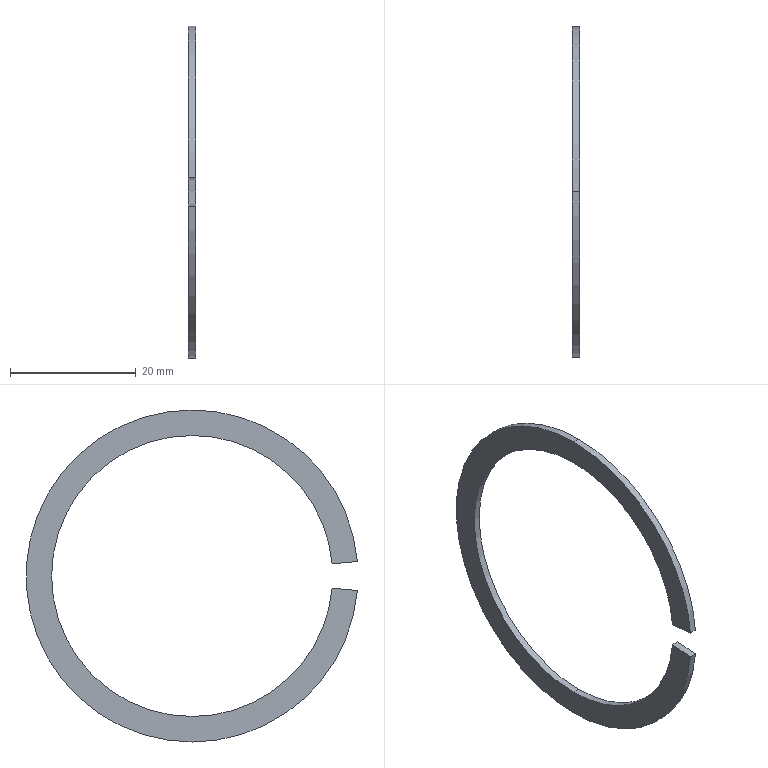Part | STEP file | 0229_Z_B6204ZZNR_2 | 1 solid | 10 faces | box 1.12 x 52.6 x 52.7 mm | volume 674.018 mm3 | cylinder 6 | plane 4 | commonest cylinder face diameters 44.6 x3 52.7 x3
STEP:
#1=CARTESIAN_POINT('',(0.,0.,0.));
#2=DIRECTION('',(0.,0.,1.));
#3=DIRECTION('',(1.,0.,0.));
#4=AXIS2_PLACEMENT_3D('',#1,#2,#3);
#5=CARTESIAN_POINT('',(3.58,-22.215,-1.944));
#6=VERTEX_POINT('',#5);
#7=CARTESIAN_POINT('',(2.46,-22.215,-1.944));
#8=VERTEX_POINT('',#7);
#9=CARTESIAN_POINT('',(2.46,-22.215,-1.944));
#10=DIRECTION('',(-1.,0.,0.));
#11=VECTOR('',#10,1.);
#12=LINE('',#9,#11);
#13=CARTESIAN_POINT('',(2.46,0.,0.));
#14=DIRECTION('',(-1.,0.,0.));
#15=DIRECTION('',(0.,0.,1.));
#16=AXIS2_PLACEMENT_3D('',#13,#14,#15);
#17=CYLINDRICAL_SURFACE('',#16,22.3);
#18=CARTESIAN_POINT('',(4.625,0.));
#19=DIRECTION('',(0.,1.));
#20=VECTOR('',#19,1.);
#21=LINE('',#18,#20);
#22=(GEOMETRIC_REPRESENTATION_CONTEXT(2)PARAMETRIC_REPRESENTATION_CONTEXT()REPRESENTATION_CONTEXT('',''));
#23=DEFINITIONAL_REPRESENTATION('',(#21),#22);
#24=PCURVE('',#17,#23);
#25=CARTESIAN_POINT('',(2.46,-26.25,-2.297));
#26=DIRECTION('',(0.,-0.08716,0.9962));
#27=DIRECTION('',(0.,-0.9962,-0.08716));
#28=AXIS2_PLACEMENT_3D('',#25,#26,#27);
#29=PLANE('',#28);
#30=CARTESIAN_POINT('',(-4.05,0.));
#31=DIRECTION('',(0.,-1.));
#32=VECTOR('',#31,1.);
#33=LINE('',#30,#32);
#34=(GEOMETRIC_REPRESENTATION_CONTEXT(2)PARAMETRIC_REPRESENTATION_CONTEXT()REPRESENTATION_CONTEXT('',''));
#35=DEFINITIONAL_REPRESENTATION('',(#33),#34);
#36=PCURVE('',#29,#35);
#37=SURFACE_CURVE('',#12,(#24,#36),.PCURVE_S1.);
#38=EDGE_CURVE('',#6,#8,#37,.T.);
#39=ORIENTED_EDGE('',*,*,#38,.T.);
#40=CARTESIAN_POINT('',(2.46,0.,-22.3));
#41=VERTEX_POINT('',#40);
#42=CARTESIAN_POINT('',(2.46,0.,0.));
#43=DIRECTION('',(1.,0.,0.));
#44=DIRECTION('',(0.,0.,1.));
#45=AXIS2_PLACEMENT_3D('',#42,#43,#44);
#46=CIRCLE('',#45,22.3);
#47=CARTESIAN_POINT('',(6.283,0.));
#48=DIRECTION('',(-1.,0.));
#49=VECTOR('',#48,1.);
#50=LINE('',#47,#49);
#51=(GEOMETRIC_REPRESENTATION_CONTEXT(2)PARAMETRIC_REPRESENTATION_CONTEXT()REPRESENTATION_CONTEXT('',''));
#52=DEFINITIONAL_REPRESENTATION('',(#50),#51);
#53=PCURVE('',#17,#52);
#54=CARTESIAN_POINT('',(2.46,0.,0.));
#55=DIRECTION('',(1.,0.,0.));
#56=DIRECTION('',(0.,0.,-1.));
#57=AXIS2_PLACEMENT_3D('',#54,#55,#56);
#58=PLANE('',#57);
#59=CARTESIAN_POINT('',(0.,0.));
#60=DIRECTION('',(-1.,0.));
#61=AXIS2_PLACEMENT_2D('',#59,#60);
#62=CIRCLE('',#61,22.3);
#63=(GEOMETRIC_REPRESENTATION_CONTEXT(2)PARAMETRIC_REPRESENTATION_CONTEXT()REPRESENTATION_CONTEXT('',''));
#64=DEFINITIONAL_REPRESENTATION('',(#62),#63);
#65=PCURVE('',#58,#64);
#66=SURFACE_CURVE('',#46,(#53,#65),.PCURVE_S1.);
#67=EDGE_CURVE('',#8,#41,#66,.T.);
#68=ORIENTED_EDGE('',*,*,#67,.T.);
#69=CARTESIAN_POINT('',(3.58,0.,-22.3));
#70=VERTEX_POINT('',#69);
#71=CARTESIAN_POINT('',(2.46,0.,-22.3));
#72=DIRECTION('',(-1.,0.,0.));
#73=VECTOR('',#72,1.);
#74=LINE('',#71,#73);
#75=CARTESIAN_POINT('',(3.142,0.));
#76=DIRECTION('',(0.,1.));
#77=VECTOR('',#76,1.);
#78=LINE('',#75,#77);
#79=(GEOMETRIC_REPRESENTATION_CONTEXT(2)PARAMETRIC_REPRESENTATION_CONTEXT()REPRESENTATION_CONTEXT('',''));
#80=DEFINITIONAL_REPRESENTATION('',(#78),#79);
#81=PCURVE('',#17,#80);
#82=CARTESIAN_POINT('',(2.46,0.,0.));
#83=DIRECTION('',(-1.,0.,0.));
#84=DIRECTION('',(0.,0.,1.));
#85=AXIS2_PLACEMENT_3D('',#82,#83,#84);
#86=CYLINDRICAL_SURFACE('',#85,22.3);
#87=CARTESIAN_POINT('',(3.142,0.));
#88=DIRECTION('',(0.,1.));
#89=VECTOR('',#88,1.);
#90=LINE('',#87,#89);
#91=(GEOMETRIC_REPRESENTATION_CONTEXT(2)PARAMETRIC_REPRESENTATION_CONTEXT()REPRESENTATION_CONTEXT('',''));
#92=DEFINITIONAL_REPRESENTATION('',(#90),#91);
#93=PCURVE('',#86,#92);
#94=SURFACE_CURVE('',#74,(#81,#93),.PCURVE_S1.);
#95=EDGE_CURVE('',#70,#41,#94,.T.);
#96=ORIENTED_EDGE('',*,*,#95,.F.);
#97=CARTESIAN_POINT('',(3.58,0.,0.));
#98=DIRECTION('',(-1.,0.,0.));
#99=DIRECTION('',(0.,0.,1.));
#100=AXIS2_PLACEMENT_3D('',#97,#98,#99);
#101=CIRCLE('',#100,22.3);
#102=CARTESIAN_POINT('',(0.,-1.12));
#103=DIRECTION('',(1.,0.));
#104=VECTOR('',#103,1.);
#105=LINE('',#102,#104);
#106=(GEOMETRIC_REPRESENTATION_CONTEXT(2)PARAMETRIC_REPRESENTATION_CONTEXT()REPRESENTATION_CONTEXT('',''));
#107=DEFINITIONAL_REPRESENTATION('',(#105),#106);
#108=PCURVE('',#17,#107);
#109=CARTESIAN_POINT('',(3.58,0.,0.));
#110=DIRECTION('',(1.,0.,0.));
#111=DIRECTION('',(0.,0.,-1.));
#112=AXIS2_PLACEMENT_3D('',#109,#110,#111);
#113=PLANE('',#112);
#114=CARTESIAN_POINT('',(-22.3,0.));
#115=CARTESIAN_POINT('',(-22.3,38.625));
#116=CARTESIAN_POINT('',(11.15,19.312));
#117=CARTESIAN_POINT('',(44.6,0.));
#118=CARTESIAN_POINT('',(11.15,-19.312));
#119=CARTESIAN_POINT('',(-22.3,-38.625));
#120=CARTESIAN_POINT('',(-22.3,0.));
#121=(BOUNDED_CURVE()B_SPLINE_CURVE(2,(#114,#115,#116,#117,#118,#119,#120),.UNSPECIFIED.,.T.,.F.)B_SPLINE_CURVE_WITH_KNOTS((1,2,2,2,2,1),(-2.094,0.,2.094,4.189,6.283,8.378),.UNSPECIFIED.)CURVE()GEOMETRIC_REPRESENTATION_ITEM()RATIONAL_B_SPLINE_CURVE((1.,0.5,1.,0.5,1.,0.5,1.))REPRESENTATION_ITEM(''));
#122=(GEOMETRIC_REPRESENTATION_CONTEXT(2)PARAMETRIC_REPRESENTATION_CONTEXT()REPRESENTATION_CONTEXT('',''));
#123=DEFINITIONAL_REPRESENTATION('',(#121),#122);
#124=PCURVE('',#113,#123);
#125=SURFACE_CURVE('',#101,(#108,#124),.PCURVE_S1.);
#126=EDGE_CURVE('',#70,#6,#125,.T.);
#127=ORIENTED_EDGE('',*,*,#126,.T.);
#128=EDGE_LOOP('',(#39,#68,#96,#127));
#129=FACE_BOUND('',#128,.F.);
#130=ADVANCED_FACE('',(#129),#17,.F.);
#131=CARTESIAN_POINT('',(2.46,0.,22.3));
#132=VERTEX_POINT('',#131);
#133=CARTESIAN_POINT('',(2.46,0.,0.));
#134=DIRECTION('',(1.,0.,0.));
#135=DIRECTION('',(0.,0.,1.));
#136=AXIS2_PLACEMENT_3D('',#133,#134,#135);
#137=CIRCLE('',#136,22.3);
#138=CARTESIAN_POINT('',(6.283,0.));
#139=DIRECTION('',(-1.,0.));
#140=VECTOR('',#139,1.);
#141=LINE('',#138,#140);
#142=(GEOMETRIC_REPRESENTATION_CONTEXT(2)PARAMETRIC_REPRESENTATION_CONTEXT()REPRESENTATION_CONTEXT('',''));
#143=DEFINITIONAL_REPRESENTATION('',(#141),#142);
#144=PCURVE('',#86,#143);
#145=CARTESIAN_POINT('',(0.,0.));
#146=DIRECTION('',(-1.,0.));
#147=AXIS2_PLACEMENT_2D('',#145,#146);
#148=CIRCLE('',#147,22.3);
#149=(GEOMETRIC_REPRESENTATION_CONTEXT(2)PARAMETRIC_REPRESENTATION_CONTEXT()REPRESENTATION_CONTEXT('',''));
#150=DEFINITIONAL_REPRESENTATION('',(#148),#149);
#151=PCURVE('',#58,#150);
#152=SURFACE_CURVE('',#137,(#144,#151),.PCURVE_S1.);
#153=EDGE_CURVE('',#41,#132,#152,.T.);
#154=ORIENTED_EDGE('',*,*,#153,.T.);
#155=CARTESIAN_POINT('',(3.58,0.,22.3));
#156=VERTEX_POINT('',#155);
#157=CARTESIAN_POINT('',(2.46,0.,22.3));
#158=DIRECTION('',(-1.,0.,0.));
#159=VECTOR('',#158,1.);
#160=LINE('',#157,#159);
#161=CARTESIAN_POINT('',(0.,0.));
#162=DIRECTION('',(0.,1.));
#163=VECTOR('',#162,1.);
#164=LINE('',#161,#163);
#165=(GEOMETRIC_REPRESENTATION_CONTEXT(2)PARAMETRIC_REPRESENTATION_CONTEXT()REPRESENTATION_CONTEXT('',''));
#166=DEFINITIONAL_REPRESENTATION('',(#164),#165);
#167=PCURVE('',#86,#166);
#168=CARTESIAN_POINT('',(2.46,0.,0.));
#169=DIRECTION('',(-1.,0.,0.));
#170=DIRECTION('',(0.,0.,1.));
#171=AXIS2_PLACEMENT_3D('',#168,#169,#170);
#172=CYLINDRICAL_SURFACE('',#171,22.3);
#173=CARTESIAN_POINT('',(6.283,0.));
#174=DIRECTION('',(0.,1.));
#175=VECTOR('',#174,1.);
#176=LINE('',#173,#175);
#177=(GEOMETRIC_REPRESENTATION_CONTEXT(2)PARAMETRIC_REPRESENTATION_CONTEXT()REPRESENTATION_CONTEXT('',''));
#178=DEFINITIONAL_REPRESENTATION('',(#176),#177);
#179=PCURVE('',#172,#178);
#180=SURFACE_CURVE('',#160,(#167,#179),.PCURVE_S1.);
#181=EDGE_CURVE('',#156,#132,#180,.T.);
#182=ORIENTED_EDGE('',*,*,#181,.F.);
#183=CARTESIAN_POINT('',(3.58,0.,0.));
#184=DIRECTION('',(-1.,0.,0.));
#185=DIRECTION('',(0.,0.,1.));
#186=AXIS2_PLACEMENT_3D('',#183,#184,#185);
#187=CIRCLE('',#186,22.3);
#188=CARTESIAN_POINT('',(0.,-1.12));
#189=DIRECTION('',(1.,0.));
#190=VECTOR('',#189,1.);
#191=LINE('',#188,#190);
#192=(GEOMETRIC_REPRESENTATION_CONTEXT(2)PARAMETRIC_REPRESENTATION_CONTEXT()REPRESENTATION_CONTEXT('',''));
#193=DEFINITIONAL_REPRESENTATION('',(#191),#192);
#194=PCURVE('',#86,#193);
#195=CARTESIAN_POINT('',(-22.3,0.));
#196=CARTESIAN_POINT('',(-22.3,38.625));
#197=CARTESIAN_POINT('',(11.15,19.312));
#198=CARTESIAN_POINT('',(44.6,0.));
#199=CARTESIAN_POINT('',(11.15,-19.312));
#200=CARTESIAN_POINT('',(-22.3,-38.625));
#201=CARTESIAN_POINT('',(-22.3,0.));
#202=(BOUNDED_CURVE()B_SPLINE_CURVE(2,(#195,#196,#197,#198,#199,#200,#201),.UNSPECIFIED.,.T.,.F.)B_SPLINE_CURVE_WITH_KNOTS((1,2,2,2,2,1),(-2.094,0.,2.094,4.189,6.283,8.378),.UNSPECIFIED.)CURVE()GEOMETRIC_REPRESENTATION_ITEM()RATIONAL_B_SPLINE_CURVE((1.,0.5,1.,0.5,1.,0.5,1.))REPRESENTATION_ITEM(''));
#203=(GEOMETRIC_REPRESENTATION_CONTEXT(2)PARAMETRIC_REPRESENTATION_CONTEXT()REPRESENTATION_CONTEXT('',''));
#204=DEFINITIONAL_REPRESENTATION('',(#202),#203);
#205=PCURVE('',#113,#204);
#206=SURFACE_CURVE('',#187,(#194,#205),.PCURVE_S1.);
#207=EDGE_CURVE('',#156,#70,#206,.T.);
#208=ORIENTED_EDGE('',*,*,#207,.T.);
#209=ORIENTED_EDGE('',*,*,#95,.T.);
#210=EDGE_LOOP('',(#154,#182,#208,#209));
#211=FACE_BOUND('',#210,.F.);
#212=ADVANCED_FACE('',(#211),#86,.F.);
#213=CARTESIAN_POINT('',(3.58,0.,-26.35));
#214=VERTEX_POINT('',#213);
#215=CARTESIAN_POINT('',(3.58,0.,26.35));
#216=VERTEX_POINT('',#215);
#217=CARTESIAN_POINT('',(3.58,0.,0.));
#218=DIRECTION('',(1.,0.,0.));
#219=DIRECTION('',(0.,0.,1.));
#220=AXIS2_PLACEMENT_3D('',#217,#218,#219);
#221=CIRCLE('',#220,26.35);
#222=CARTESIAN_POINT('',(2.46,0.,0.));
#223=DIRECTION('',(-1.,0.,0.));
#224=DIRECTION('',(0.,0.,1.));
#225=AXIS2_PLACEMENT_3D('',#222,#223,#224);
#226=CYLINDRICAL_SURFACE('',#225,26.35);
#227=CARTESIAN_POINT('',(6.283,-1.12));
#228=DIRECTION('',(-1.,0.));
#229=VECTOR('',#228,1.);
#230=LINE('',#227,#229);
#231=(GEOMETRIC_REPRESENTATION_CONTEXT(2)PARAMETRIC_REPRESENTATION_CONTEXT()REPRESENTATION_CONTEXT('',''));
#232=DEFINITIONAL_REPRESENTATION('',(#230),#231);
#233=PCURVE('',#226,#232);
#234=CARTESIAN_POINT('',(0.,0.));
#235=DIRECTION('',(-1.,0.));
#236=AXIS2_PLACEMENT_2D('',#234,#235);
#237=CIRCLE('',#236,26.35);
#238=(GEOMETRIC_REPRESENTATION_CONTEXT(2)PARAMETRIC_REPRESENTATION_CONTEXT()REPRESENTATION_CONTEXT('',''));
#239=DEFINITIONAL_REPRESENTATION('',(#237),#238);
#240=PCURVE('',#113,#239);
#241=SURFACE_CURVE('',#221,(#233,#240),.PCURVE_S1.);
#242=EDGE_CURVE('',#214,#216,#241,.T.);
#243=ORIENTED_EDGE('',*,*,#242,.F.);
#244=CARTESIAN_POINT('',(2.46,0.,-26.35));
#245=VERTEX_POINT('',#244);
#246=CARTESIAN_POINT('',(2.46,0.,-26.35));
#247=DIRECTION('',(-1.,0.,0.));
#248=VECTOR('',#247,1.);
#249=LINE('',#246,#248);
#250=CARTESIAN_POINT('',(3.142,0.));
#251=DIRECTION('',(0.,1.));
#252=VECTOR('',#251,1.);
#253=LINE('',#250,#252);
#254=(GEOMETRIC_REPRESENTATION_CONTEXT(2)PARAMETRIC_REPRESENTATION_CONTEXT()REPRESENTATION_CONTEXT('',''));
#255=DEFINITIONAL_REPRESENTATION('',(#253),#254);
#256=PCURVE('',#226,#255);
#257=CARTESIAN_POINT('',(2.46,0.,0.));
#258=DIRECTION('',(-1.,0.,0.));
#259=DIRECTION('',(0.,0.,1.));
#260=AXIS2_PLACEMENT_3D('',#257,#258,#259);
#261=CYLINDRICAL_SURFACE('',#260,26.35);
#262=CARTESIAN_POINT('',(3.142,0.));
#263=DIRECTION('',(0.,1.));
#264=VECTOR('',#263,1.);
#265=LINE('',#262,#264);
#266=(GEOMETRIC_REPRESENTATION_CONTEXT(2)PARAMETRIC_REPRESENTATION_CONTEXT()REPRESENTATION_CONTEXT('',''));
#267=DEFINITIONAL_REPRESENTATION('',(#265),#266);
#268=PCURVE('',#261,#267);
#269=SURFACE_CURVE('',#249,(#256,#268),.PCURVE_S1.);
#270=EDGE_CURVE('',#214,#245,#269,.T.);
#271=ORIENTED_EDGE('',*,*,#270,.T.);
#272=CARTESIAN_POINT('',(2.46,0.,26.35));
#273=VERTEX_POINT('',#272);
#274=CARTESIAN_POINT('',(2.46,0.,0.));
#275=DIRECTION('',(1.,0.,0.));
#276=DIRECTION('',(0.,0.,1.));
#277=AXIS2_PLACEMENT_3D('',#274,#275,#276);
#278=CIRCLE('',#277,26.35);
#279=CARTESIAN_POINT('',(6.283,0.));
#280=DIRECTION('',(-1.,0.));
#281=VECTOR('',#280,1.);
#282=LINE('',#279,#281);
#283=(GEOMETRIC_REPRESENTATION_CONTEXT(2)PARAMETRIC_REPRESENTATION_CONTEXT()REPRESENTATION_CONTEXT('',''));
#284=DEFINITIONAL_REPRESENTATION('',(#282),#283);
#285=PCURVE('',#226,#284);
#286=CARTESIAN_POINT('',(0.,0.));
#287=DIRECTION('',(-1.,0.));
#288=AXIS2_PLACEMENT_2D('',#286,#287);
#289=CIRCLE('',#288,26.35);
#290=(GEOMETRIC_REPRESENTATION_CONTEXT(2)PARAMETRIC_REPRESENTATION_CONTEXT()REPRESENTATION_CONTEXT('',''));
#291=DEFINITIONAL_REPRESENTATION('',(#289),#290);
#292=PCURVE('',#58,#291);
#293=SURFACE_CURVE('',#278,(#285,#292),.PCURVE_S1.);
#294=EDGE_CURVE('',#245,#273,#293,.T.);
#295=ORIENTED_EDGE('',*,*,#294,.T.);
#296=CARTESIAN_POINT('',(2.46,0.,26.35));
#297=DIRECTION('',(-1.,0.,0.));
#298=VECTOR('',#297,1.);
#299=LINE('',#296,#298);
#300=CARTESIAN_POINT('',(0.,0.));
#301=DIRECTION('',(0.,1.));
#302=VECTOR('',#301,1.);
#303=LINE('',#300,#302);
#304=(GEOMETRIC_REPRESENTATION_CONTEXT(2)PARAMETRIC_REPRESENTATION_CONTEXT()REPRESENTATION_CONTEXT('',''));
#305=DEFINITIONAL_REPRESENTATION('',(#303),#304);
#306=PCURVE('',#226,#305);
#307=CARTESIAN_POINT('',(2.46,0.,0.));
#308=DIRECTION('',(-1.,0.,0.));
#309=DIRECTION('',(0.,0.,1.));
#310=AXIS2_PLACEMENT_3D('',#307,#308,#309);
#311=CYLINDRICAL_SURFACE('',#310,26.35);
#312=CARTESIAN_POINT('',(6.283,0.));
#313=DIRECTION('',(0.,1.));
#314=VECTOR('',#313,1.);
#315=LINE('',#312,#314);
#316=(GEOMETRIC_REPRESENTATION_CONTEXT(2)PARAMETRIC_REPRESENTATION_CONTEXT()REPRESENTATION_CONTEXT('',''));
#317=DEFINITIONAL_REPRESENTATION('',(#315),#316);
#318=PCURVE('',#311,#317);
#319=SURFACE_CURVE('',#299,(#306,#318),.PCURVE_S1.);
#320=EDGE_CURVE('',#216,#273,#319,.T.);
#321=ORIENTED_EDGE('',*,*,#320,.F.);
#322=EDGE_LOOP('',(#243,#271,#295,#321));
#323=FACE_BOUND('',#322,.T.);
#324=ADVANCED_FACE('',(#323),#226,.T.);
#325=CARTESIAN_POINT('',(3.58,-26.25,2.297));
#326=VERTEX_POINT('',#325);
#327=CARTESIAN_POINT('',(3.58,0.,0.));
#328=DIRECTION('',(1.,0.,0.));
#329=DIRECTION('',(0.,0.,1.));
#330=AXIS2_PLACEMENT_3D('',#327,#328,#329);
#331=CIRCLE('',#330,26.35);
#332=CARTESIAN_POINT('',(6.283,-1.12));
#333=DIRECTION('',(-1.,0.));
#334=VECTOR('',#333,1.);
#335=LINE('',#332,#334);
#336=(GEOMETRIC_REPRESENTATION_CONTEXT(2)PARAMETRIC_REPRESENTATION_CONTEXT()REPRESENTATION_CONTEXT('',''));
#337=DEFINITIONAL_REPRESENTATION('',(#335),#336);
#338=PCURVE('',#311,#337);
#339=CARTESIAN_POINT('',(0.,0.));
#340=DIRECTION('',(-1.,0.));
#341=AXIS2_PLACEMENT_2D('',#339,#340);
#342=CIRCLE('',#341,26.35);
#343=(GEOMETRIC_REPRESENTATION_CONTEXT(2)PARAMETRIC_REPRESENTATION_CONTEXT()REPRESENTATION_CONTEXT('',''));
#344=DEFINITIONAL_REPRESENTATION('',(#342),#343);
#345=PCURVE('',#113,#344);
#346=SURFACE_CURVE('',#331,(#338,#345),.PCURVE_S1.);
#347=EDGE_CURVE('',#216,#326,#346,.T.);
#348=ORIENTED_EDGE('',*,*,#347,.F.);
#349=ORIENTED_EDGE('',*,*,#320,.T.);
#350=CARTESIAN_POINT('',(2.46,-26.25,2.297));
#351=VERTEX_POINT('',#350);
#352=CARTESIAN_POINT('',(2.46,0.,0.));
#353=DIRECTION('',(1.,0.,0.));
#354=DIRECTION('',(0.,0.,1.));
#355=AXIS2_PLACEMENT_3D('',#352,#353,#354);
#356=CIRCLE('',#355,26.35);
#357=CARTESIAN_POINT('',(6.283,0.));
#358=DIRECTION('',(-1.,0.));
#359=VECTOR('',#358,1.);
#360=LINE('',#357,#359);
#361=(GEOMETRIC_REPRESENTATION_CONTEXT(2)PARAMETRIC_REPRESENTATION_CONTEXT()REPRESENTATION_CONTEXT('',''));
#362=DEFINITIONAL_REPRESENTATION('',(#360),#361);
#363=PCURVE('',#311,#362);
#364=CARTESIAN_POINT('',(0.,0.));
#365=DIRECTION('',(-1.,0.));
#366=AXIS2_PLACEMENT_2D('',#364,#365);
#367=CIRCLE('',#366,26.35);
#368=(GEOMETRIC_REPRESENTATION_CONTEXT(2)PARAMETRIC_REPRESENTATION_CONTEXT()REPRESENTATION_CONTEXT('',''));
#369=DEFINITIONAL_REPRESENTATION('',(#367),#368);
#370=PCURVE('',#58,#369);
#371=SURFACE_CURVE('',#356,(#363,#370),.PCURVE_S1.);
#372=EDGE_CURVE('',#273,#351,#371,.T.);
#373=ORIENTED_EDGE('',*,*,#372,.T.);
#374=CARTESIAN_POINT('',(2.46,-26.25,2.297));
#375=DIRECTION('',(-1.,0.,0.));
#376=VECTOR('',#375,1.);
#377=LINE('',#374,#376);
#378=CARTESIAN_POINT('',(4.8,0.));
#379=DIRECTION('',(0.,1.));
#380=VECTOR('',#379,1.);
#381=LINE('',#378,#380);
#382=(GEOMETRIC_REPRESENTATION_CONTEXT(2)PARAMETRIC_REPRESENTATION_CONTEXT()REPRESENTATION_CONTEXT('',''));
#383=DEFINITIONAL_REPRESENTATION('',(#381),#382);
#384=PCURVE('',#311,#383);
#385=CARTESIAN_POINT('',(2.46,-22.215,1.944));
#386=DIRECTION('',(0.,-0.08716,-0.9962));
#387=DIRECTION('',(0.,0.9962,-0.08716));
#388=AXIS2_PLACEMENT_3D('',#385,#386,#387);
#389=PLANE('',#388);
#390=CARTESIAN_POINT('',(-4.05,0.));
#391=DIRECTION('',(0.,-1.));
#392=VECTOR('',#391,1.);
#393=LINE('',#390,#392);
#394=(GEOMETRIC_REPRESENTATION_CONTEXT(2)PARAMETRIC_REPRESENTATION_CONTEXT()REPRESENTATION_CONTEXT('',''));
#395=DEFINITIONAL_REPRESENTATION('',(#393),#394);
#396=PCURVE('',#389,#395);
#397=SURFACE_CURVE('',#377,(#384,#396),.PCURVE_S1.);
#398=EDGE_CURVE('',#326,#351,#397,.T.);
#399=ORIENTED_EDGE('',*,*,#398,.F.);
#400=EDGE_LOOP('',(#348,#349,#373,#399));
#401=FACE_BOUND('',#400,.T.);
#402=ADVANCED_FACE('',(#401),#311,.T.);
#403=CARTESIAN_POINT('',(3.58,-22.215,1.944));
#404=VERTEX_POINT('',#403);
#405=CARTESIAN_POINT('',(3.58,0.,0.));
#406=DIRECTION('',(-1.,0.,0.));
#407=DIRECTION('',(0.,0.,1.));
#408=AXIS2_PLACEMENT_3D('',#405,#406,#407);
#409=CIRCLE('',#408,22.3);
#410=CARTESIAN_POINT('',(-22.3,0.));
#411=CARTESIAN_POINT('',(-22.3,38.625));
#412=CARTESIAN_POINT('',(11.15,19.312));
#413=CARTESIAN_POINT('',(44.6,0.));
#414=CARTESIAN_POINT('',(11.15,-19.312));
#415=CARTESIAN_POINT('',(-22.3,-38.625));
#416=CARTESIAN_POINT('',(-22.3,0.));
#417=(BOUNDED_CURVE()B_SPLINE_CURVE(2,(#410,#411,#412,#413,#414,#415,#416),.UNSPECIFIED.,.T.,.F.)B_SPLINE_CURVE_WITH_KNOTS((1,2,2,2,2,1),(-2.094,0.,2.094,4.189,6.283,8.378),.UNSPECIFIED.)CURVE()GEOMETRIC_REPRESENTATION_ITEM()RATIONAL_B_SPLINE_CURVE((1.,0.5,1.,0.5,1.,0.5,1.))REPRESENTATION_ITEM(''));
#418=(GEOMETRIC_REPRESENTATION_CONTEXT(2)PARAMETRIC_REPRESENTATION_CONTEXT()REPRESENTATION_CONTEXT('',''));
#419=DEFINITIONAL_REPRESENTATION('',(#417),#418);
#420=PCURVE('',#113,#419);
#421=CARTESIAN_POINT('',(0.,-1.12));
#422=DIRECTION('',(1.,0.));
#423=VECTOR('',#422,1.);
#424=LINE('',#421,#423);
#425=(GEOMETRIC_REPRESENTATION_CONTEXT(2)PARAMETRIC_REPRESENTATION_CONTEXT()REPRESENTATION_CONTEXT('',''));
#426=DEFINITIONAL_REPRESENTATION('',(#424),#425);
#427=PCURVE('',#172,#426);
#428=SURFACE_CURVE('',#409,(#420,#427),.PCURVE_S1.);
#429=EDGE_CURVE('',#404,#156,#428,.T.);
#430=ORIENTED_EDGE('',*,*,#429,.T.);
#431=ORIENTED_EDGE('',*,*,#207,.T.);
#432=ORIENTED_EDGE('',*,*,#126,.T.);
#433=CARTESIAN_POINT('',(3.58,-26.25,-2.297));
#434=VERTEX_POINT('',#433);
#435=CARTESIAN_POINT('',(3.58,-22.215,-1.944));
#436=DIRECTION('',(0.,-0.9962,-0.08716));
#437=VECTOR('',#436,1.);
#438=LINE('',#435,#437);
#439=CARTESIAN_POINT('',(1.944,-22.215));
#440=DIRECTION('',(0.08716,-0.9962));
#441=VECTOR('',#440,1.);
#442=LINE('',#439,#441);
#443=(GEOMETRIC_REPRESENTATION_CONTEXT(2)PARAMETRIC_REPRESENTATION_CONTEXT()REPRESENTATION_CONTEXT('',''));
#444=DEFINITIONAL_REPRESENTATION('',(#442),#443);
#445=PCURVE('',#113,#444);
#446=CARTESIAN_POINT('',(-4.05,1.12));
#447=DIRECTION('',(1.,0.));
#448=VECTOR('',#447,1.);
#449=LINE('',#446,#448);
#450=(GEOMETRIC_REPRESENTATION_CONTEXT(2)PARAMETRIC_REPRESENTATION_CONTEXT()REPRESENTATION_CONTEXT('',''));
#451=DEFINITIONAL_REPRESENTATION('',(#449),#450);
#452=PCURVE('',#29,#451);
#453=SURFACE_CURVE('',#438,(#445,#452),.PCURVE_S1.);
#454=EDGE_CURVE('',#6,#434,#453,.T.);
#455=ORIENTED_EDGE('',*,*,#454,.T.);
#456=CARTESIAN_POINT('',(3.58,0.,0.));
#457=DIRECTION('',(1.,0.,0.));
#458=DIRECTION('',(0.,0.,1.));
#459=AXIS2_PLACEMENT_3D('',#456,#457,#458);
#460=CIRCLE('',#459,26.35);
#461=CARTESIAN_POINT('',(0.,0.));
#462=DIRECTION('',(-1.,0.));
#463=AXIS2_PLACEMENT_2D('',#461,#462);
#464=CIRCLE('',#463,26.35);
#465=(GEOMETRIC_REPRESENTATION_CONTEXT(2)PARAMETRIC_REPRESENTATION_CONTEXT()REPRESENTATION_CONTEXT('',''));
#466=DEFINITIONAL_REPRESENTATION('',(#464),#465);
#467=PCURVE('',#113,#466);
#468=CARTESIAN_POINT('',(6.283,-1.12));
#469=DIRECTION('',(-1.,0.));
#470=VECTOR('',#469,1.);
#471=LINE('',#468,#470);
#472=(GEOMETRIC_REPRESENTATION_CONTEXT(2)PARAMETRIC_REPRESENTATION_CONTEXT()REPRESENTATION_CONTEXT('',''));
#473=DEFINITIONAL_REPRESENTATION('',(#471),#472);
#474=PCURVE('',#261,#473);
#475=SURFACE_CURVE('',#460,(#467,#474),.PCURVE_S1.);
#476=EDGE_CURVE('',#434,#214,#475,.T.);
#477=ORIENTED_EDGE('',*,*,#476,.T.);
#478=ORIENTED_EDGE('',*,*,#242,.T.);
#479=ORIENTED_EDGE('',*,*,#347,.T.);
#480=CARTESIAN_POINT('',(3.58,-26.25,2.297));
#481=DIRECTION('',(0.,0.9962,-0.08716));
#482=VECTOR('',#481,1.);
#483=LINE('',#480,#482);
#484=CARTESIAN_POINT('',(-2.297,-26.25));
#485=DIRECTION('',(0.08716,0.9962));
#486=VECTOR('',#485,1.);
#487=LINE('',#484,#486);
#488=(GEOMETRIC_REPRESENTATION_CONTEXT(2)PARAMETRIC_REPRESENTATION_CONTEXT()REPRESENTATION_CONTEXT('',''));
#489=DEFINITIONAL_REPRESENTATION('',(#487),#488);
#490=PCURVE('',#113,#489);
#491=CARTESIAN_POINT('',(-4.05,1.12));
#492=DIRECTION('',(1.,0.));
#493=VECTOR('',#492,1.);
#494=LINE('',#491,#493);
#495=(GEOMETRIC_REPRESENTATION_CONTEXT(2)PARAMETRIC_REPRESENTATION_CONTEXT()REPRESENTATION_CONTEXT('',''));
#496=DEFINITIONAL_REPRESENTATION('',(#494),#495);
#497=PCURVE('',#389,#496);
#498=SURFACE_CURVE('',#483,(#490,#497),.PCURVE_S1.);
#499=EDGE_CURVE('',#326,#404,#498,.T.);
#500=ORIENTED_EDGE('',*,*,#499,.T.);
#501=EDGE_LOOP('',(#430,#431,#432,#455,#477,#478,#479,#500));
#502=FACE_BOUND('',#501,.T.);
#503=ADVANCED_FACE('',(#502),#113,.T.);
#504=CARTESIAN_POINT('',(2.46,-22.215,1.944));
#505=VERTEX_POINT('',#504);
#506=CARTESIAN_POINT('',(2.46,0.,0.));
#507=DIRECTION('',(1.,0.,0.));
#508=DIRECTION('',(0.,0.,1.));
#509=AXIS2_PLACEMENT_3D('',#506,#507,#508);
#510=CIRCLE('',#509,22.3);
#511=CARTESIAN_POINT('',(6.283,0.));
#512=DIRECTION('',(-1.,0.));
#513=VECTOR('',#512,1.);
#514=LINE('',#511,#513);
#515=(GEOMETRIC_REPRESENTATION_CONTEXT(2)PARAMETRIC_REPRESENTATION_CONTEXT()REPRESENTATION_CONTEXT('',''));
#516=DEFINITIONAL_REPRESENTATION('',(#514),#515);
#517=PCURVE('',#172,#516);
#518=CARTESIAN_POINT('',(0.,0.));
#519=DIRECTION('',(-1.,0.));
#520=AXIS2_PLACEMENT_2D('',#518,#519);
#521=CIRCLE('',#520,22.3);
#522=(GEOMETRIC_REPRESENTATION_CONTEXT(2)PARAMETRIC_REPRESENTATION_CONTEXT()REPRESENTATION_CONTEXT('',''));
#523=DEFINITIONAL_REPRESENTATION('',(#521),#522);
#524=PCURVE('',#58,#523);
#525=SURFACE_CURVE('',#510,(#517,#524),.PCURVE_S1.);
#526=EDGE_CURVE('',#132,#505,#525,.T.);
#527=ORIENTED_EDGE('',*,*,#526,.T.);
#528=CARTESIAN_POINT('',(2.46,-22.215,1.944));
#529=DIRECTION('',(1.,0.,0.));
#530=VECTOR('',#529,1.);
#531=LINE('',#528,#530);
#532=CARTESIAN_POINT('',(4.8,0.));
#533=DIRECTION('',(0.,-1.));
#534=VECTOR('',#533,1.);
#535=LINE('',#532,#534);
#536=(GEOMETRIC_REPRESENTATION_CONTEXT(2)PARAMETRIC_REPRESENTATION_CONTEXT()REPRESENTATION_CONTEXT('',''));
#537=DEFINITIONAL_REPRESENTATION('',(#535),#536);
#538=PCURVE('',#172,#537);
#539=CARTESIAN_POINT('',(0.,0.));
#540=DIRECTION('',(0.,1.));
#541=VECTOR('',#540,1.);
#542=LINE('',#539,#541);
#543=(GEOMETRIC_REPRESENTATION_CONTEXT(2)PARAMETRIC_REPRESENTATION_CONTEXT()REPRESENTATION_CONTEXT('',''));
#544=DEFINITIONAL_REPRESENTATION('',(#542),#543);
#545=PCURVE('',#389,#544);
#546=SURFACE_CURVE('',#531,(#538,#545),.PCURVE_S1.);
#547=EDGE_CURVE('',#505,#404,#546,.T.);
#548=ORIENTED_EDGE('',*,*,#547,.T.);
#549=ORIENTED_EDGE('',*,*,#429,.T.);
#550=ORIENTED_EDGE('',*,*,#181,.T.);
#551=EDGE_LOOP('',(#527,#548,#549,#550));
#552=FACE_BOUND('',#551,.F.);
#553=ADVANCED_FACE('',(#552),#172,.F.);
#554=CARTESIAN_POINT('',(2.46,-22.215,1.944));
#555=DIRECTION('',(0.,0.9962,-0.08716));
#556=VECTOR('',#555,1.);
#557=LINE('',#554,#556);
#558=CARTESIAN_POINT('',(0.,0.));
#559=DIRECTION('',(1.,0.));
#560=VECTOR('',#559,1.);
#561=LINE('',#558,#560);
#562=(GEOMETRIC_REPRESENTATION_CONTEXT(2)PARAMETRIC_REPRESENTATION_CONTEXT()REPRESENTATION_CONTEXT('',''));
#563=DEFINITIONAL_REPRESENTATION('',(#561),#562);
#564=PCURVE('',#389,#563);
#565=CARTESIAN_POINT('',(-1.944,-22.215));
#566=DIRECTION('',(0.08716,0.9962));
#567=VECTOR('',#566,1.);
#568=LINE('',#565,#567);
#569=(GEOMETRIC_REPRESENTATION_CONTEXT(2)PARAMETRIC_REPRESENTATION_CONTEXT()REPRESENTATION_CONTEXT('',''));
#570=DEFINITIONAL_REPRESENTATION('',(#568),#569);
#571=PCURVE('',#58,#570);
#572=SURFACE_CURVE('',#557,(#564,#571),.PCURVE_S1.);
#573=EDGE_CURVE('',#351,#505,#572,.T.);
#574=ORIENTED_EDGE('',*,*,#573,.T.);
#575=ORIENTED_EDGE('',*,*,#547,.T.);
#576=ORIENTED_EDGE('',*,*,#499,.F.);
#577=ORIENTED_EDGE('',*,*,#398,.T.);
#578=EDGE_LOOP('',(#574,#575,#576,#577));
#579=FACE_BOUND('',#578,.T.);
#580=ADVANCED_FACE('',(#579),#389,.T.);
#581=ORIENTED_EDGE('',*,*,#270,.F.);
#582=ORIENTED_EDGE('',*,*,#476,.F.);
#583=CARTESIAN_POINT('',(2.46,-26.25,-2.297));
#584=VERTEX_POINT('',#583);
#585=CARTESIAN_POINT('',(2.46,-26.25,-2.297));
#586=DIRECTION('',(-1.,0.,0.));
#587=VECTOR('',#586,1.);
#588=LINE('',#585,#587);
#589=CARTESIAN_POINT('',(4.625,0.));
#590=DIRECTION('',(0.,1.));
#591=VECTOR('',#590,1.);
#592=LINE('',#589,#591);
#593=(GEOMETRIC_REPRESENTATION_CONTEXT(2)PARAMETRIC_REPRESENTATION_CONTEXT()REPRESENTATION_CONTEXT('',''));
#594=DEFINITIONAL_REPRESENTATION('',(#592),#593);
#595=PCURVE('',#261,#594);
#596=CARTESIAN_POINT('',(0.,0.));
#597=DIRECTION('',(0.,-1.));
#598=VECTOR('',#597,1.);
#599=LINE('',#596,#598);
#600=(GEOMETRIC_REPRESENTATION_CONTEXT(2)PARAMETRIC_REPRESENTATION_CONTEXT()REPRESENTATION_CONTEXT('',''));
#601=DEFINITIONAL_REPRESENTATION('',(#599),#600);
#602=PCURVE('',#29,#601);
#603=SURFACE_CURVE('',#588,(#595,#602),.PCURVE_S1.);
#604=EDGE_CURVE('',#434,#584,#603,.T.);
#605=ORIENTED_EDGE('',*,*,#604,.T.);
#606=CARTESIAN_POINT('',(2.46,0.,0.));
#607=DIRECTION('',(1.,0.,0.));
#608=DIRECTION('',(0.,0.,1.));
#609=AXIS2_PLACEMENT_3D('',#606,#607,#608);
#610=CIRCLE('',#609,26.35);
#611=CARTESIAN_POINT('',(6.283,0.));
#612=DIRECTION('',(-1.,0.));
#613=VECTOR('',#612,1.);
#614=LINE('',#611,#613);
#615=(GEOMETRIC_REPRESENTATION_CONTEXT(2)PARAMETRIC_REPRESENTATION_CONTEXT()REPRESENTATION_CONTEXT('',''));
#616=DEFINITIONAL_REPRESENTATION('',(#614),#615);
#617=PCURVE('',#261,#616);
#618=CARTESIAN_POINT('',(0.,0.));
#619=DIRECTION('',(-1.,0.));
#620=AXIS2_PLACEMENT_2D('',#618,#619);
#621=CIRCLE('',#620,26.35);
#622=(GEOMETRIC_REPRESENTATION_CONTEXT(2)PARAMETRIC_REPRESENTATION_CONTEXT()REPRESENTATION_CONTEXT('',''));
#623=DEFINITIONAL_REPRESENTATION('',(#621),#622);
#624=PCURVE('',#58,#623);
#625=SURFACE_CURVE('',#610,(#617,#624),.PCURVE_S1.);
#626=EDGE_CURVE('',#584,#245,#625,.T.);
#627=ORIENTED_EDGE('',*,*,#626,.T.);
#628=EDGE_LOOP('',(#581,#582,#605,#627));
#629=FACE_BOUND('',#628,.T.);
#630=ADVANCED_FACE('',(#629),#261,.T.);
#631=CARTESIAN_POINT('',(2.46,-26.25,-2.297));
#632=DIRECTION('',(0.,-0.9962,-0.08716));
#633=VECTOR('',#632,1.);
#634=LINE('',#631,#633);
#635=CARTESIAN_POINT('',(0.,0.));
#636=DIRECTION('',(1.,0.));
#637=VECTOR('',#636,1.);
#638=LINE('',#635,#637);
#639=(GEOMETRIC_REPRESENTATION_CONTEXT(2)PARAMETRIC_REPRESENTATION_CONTEXT()REPRESENTATION_CONTEXT('',''));
#640=DEFINITIONAL_REPRESENTATION('',(#638),#639);
#641=PCURVE('',#29,#640);
#642=CARTESIAN_POINT('',(2.297,-26.25));
#643=DIRECTION('',(0.08716,-0.9962));
#644=VECTOR('',#643,1.);
#645=LINE('',#642,#644);
#646=(GEOMETRIC_REPRESENTATION_CONTEXT(2)PARAMETRIC_REPRESENTATION_CONTEXT()REPRESENTATION_CONTEXT('',''));
#647=DEFINITIONAL_REPRESENTATION('',(#645),#646);
#648=PCURVE('',#58,#647);
#649=SURFACE_CURVE('',#634,(#641,#648),.PCURVE_S1.);
#650=EDGE_CURVE('',#8,#584,#649,.T.);
#651=ORIENTED_EDGE('',*,*,#650,.T.);
#652=ORIENTED_EDGE('',*,*,#604,.F.);
#653=ORIENTED_EDGE('',*,*,#454,.F.);
#654=ORIENTED_EDGE('',*,*,#38,.T.);
#655=EDGE_LOOP('',(#651,#652,#653,#654));
#656=FACE_BOUND('',#655,.T.);
#657=ADVANCED_FACE('',(#656),#29,.T.);
#658=ORIENTED_EDGE('',*,*,#650,.F.);
#659=ORIENTED_EDGE('',*,*,#67,.T.);
#660=ORIENTED_EDGE('',*,*,#153,.T.);
#661=ORIENTED_EDGE('',*,*,#526,.T.);
#662=ORIENTED_EDGE('',*,*,#573,.F.);
#663=ORIENTED_EDGE('',*,*,#372,.F.);
#664=ORIENTED_EDGE('',*,*,#294,.F.);
#665=ORIENTED_EDGE('',*,*,#626,.F.);
#666=EDGE_LOOP('',(#658,#659,#660,#661,#662,#663,#664,#665));
#667=FACE_BOUND('',#666,.T.);
#668=ADVANCED_FACE('',(#667),#58,.F.);
#669=CLOSED_SHELL('',(#130,#212,#324,#402,#503,#553,#580,#630,#657,#668));
#670=MANIFOLD_SOLID_BREP('',#669);
#671=(LENGTH_UNIT()NAMED_UNIT(*)SI_UNIT(.MILLI.,.METRE.));
#672=UNCERTAINTY_MEASURE_WITH_UNIT(LENGTH_MEASURE(0.0000001),#671,'','');
#673=(NAMED_UNIT(*)PLANE_ANGLE_UNIT()SI_UNIT($,.RADIAN.));
#674=(NAMED_UNIT(*)SI_UNIT($,.STERADIAN.)SOLID_ANGLE_UNIT());
#675=(GEOMETRIC_REPRESENTATION_CONTEXT(3)GLOBAL_UNCERTAINTY_ASSIGNED_CONTEXT((#672))GLOBAL_UNIT_ASSIGNED_CONTEXT((#671,#673,#674))REPRESENTATION_CONTEXT('',''));
#676=ADVANCED_BREP_SHAPE_REPRESENTATION('',(#4,#670),#675);